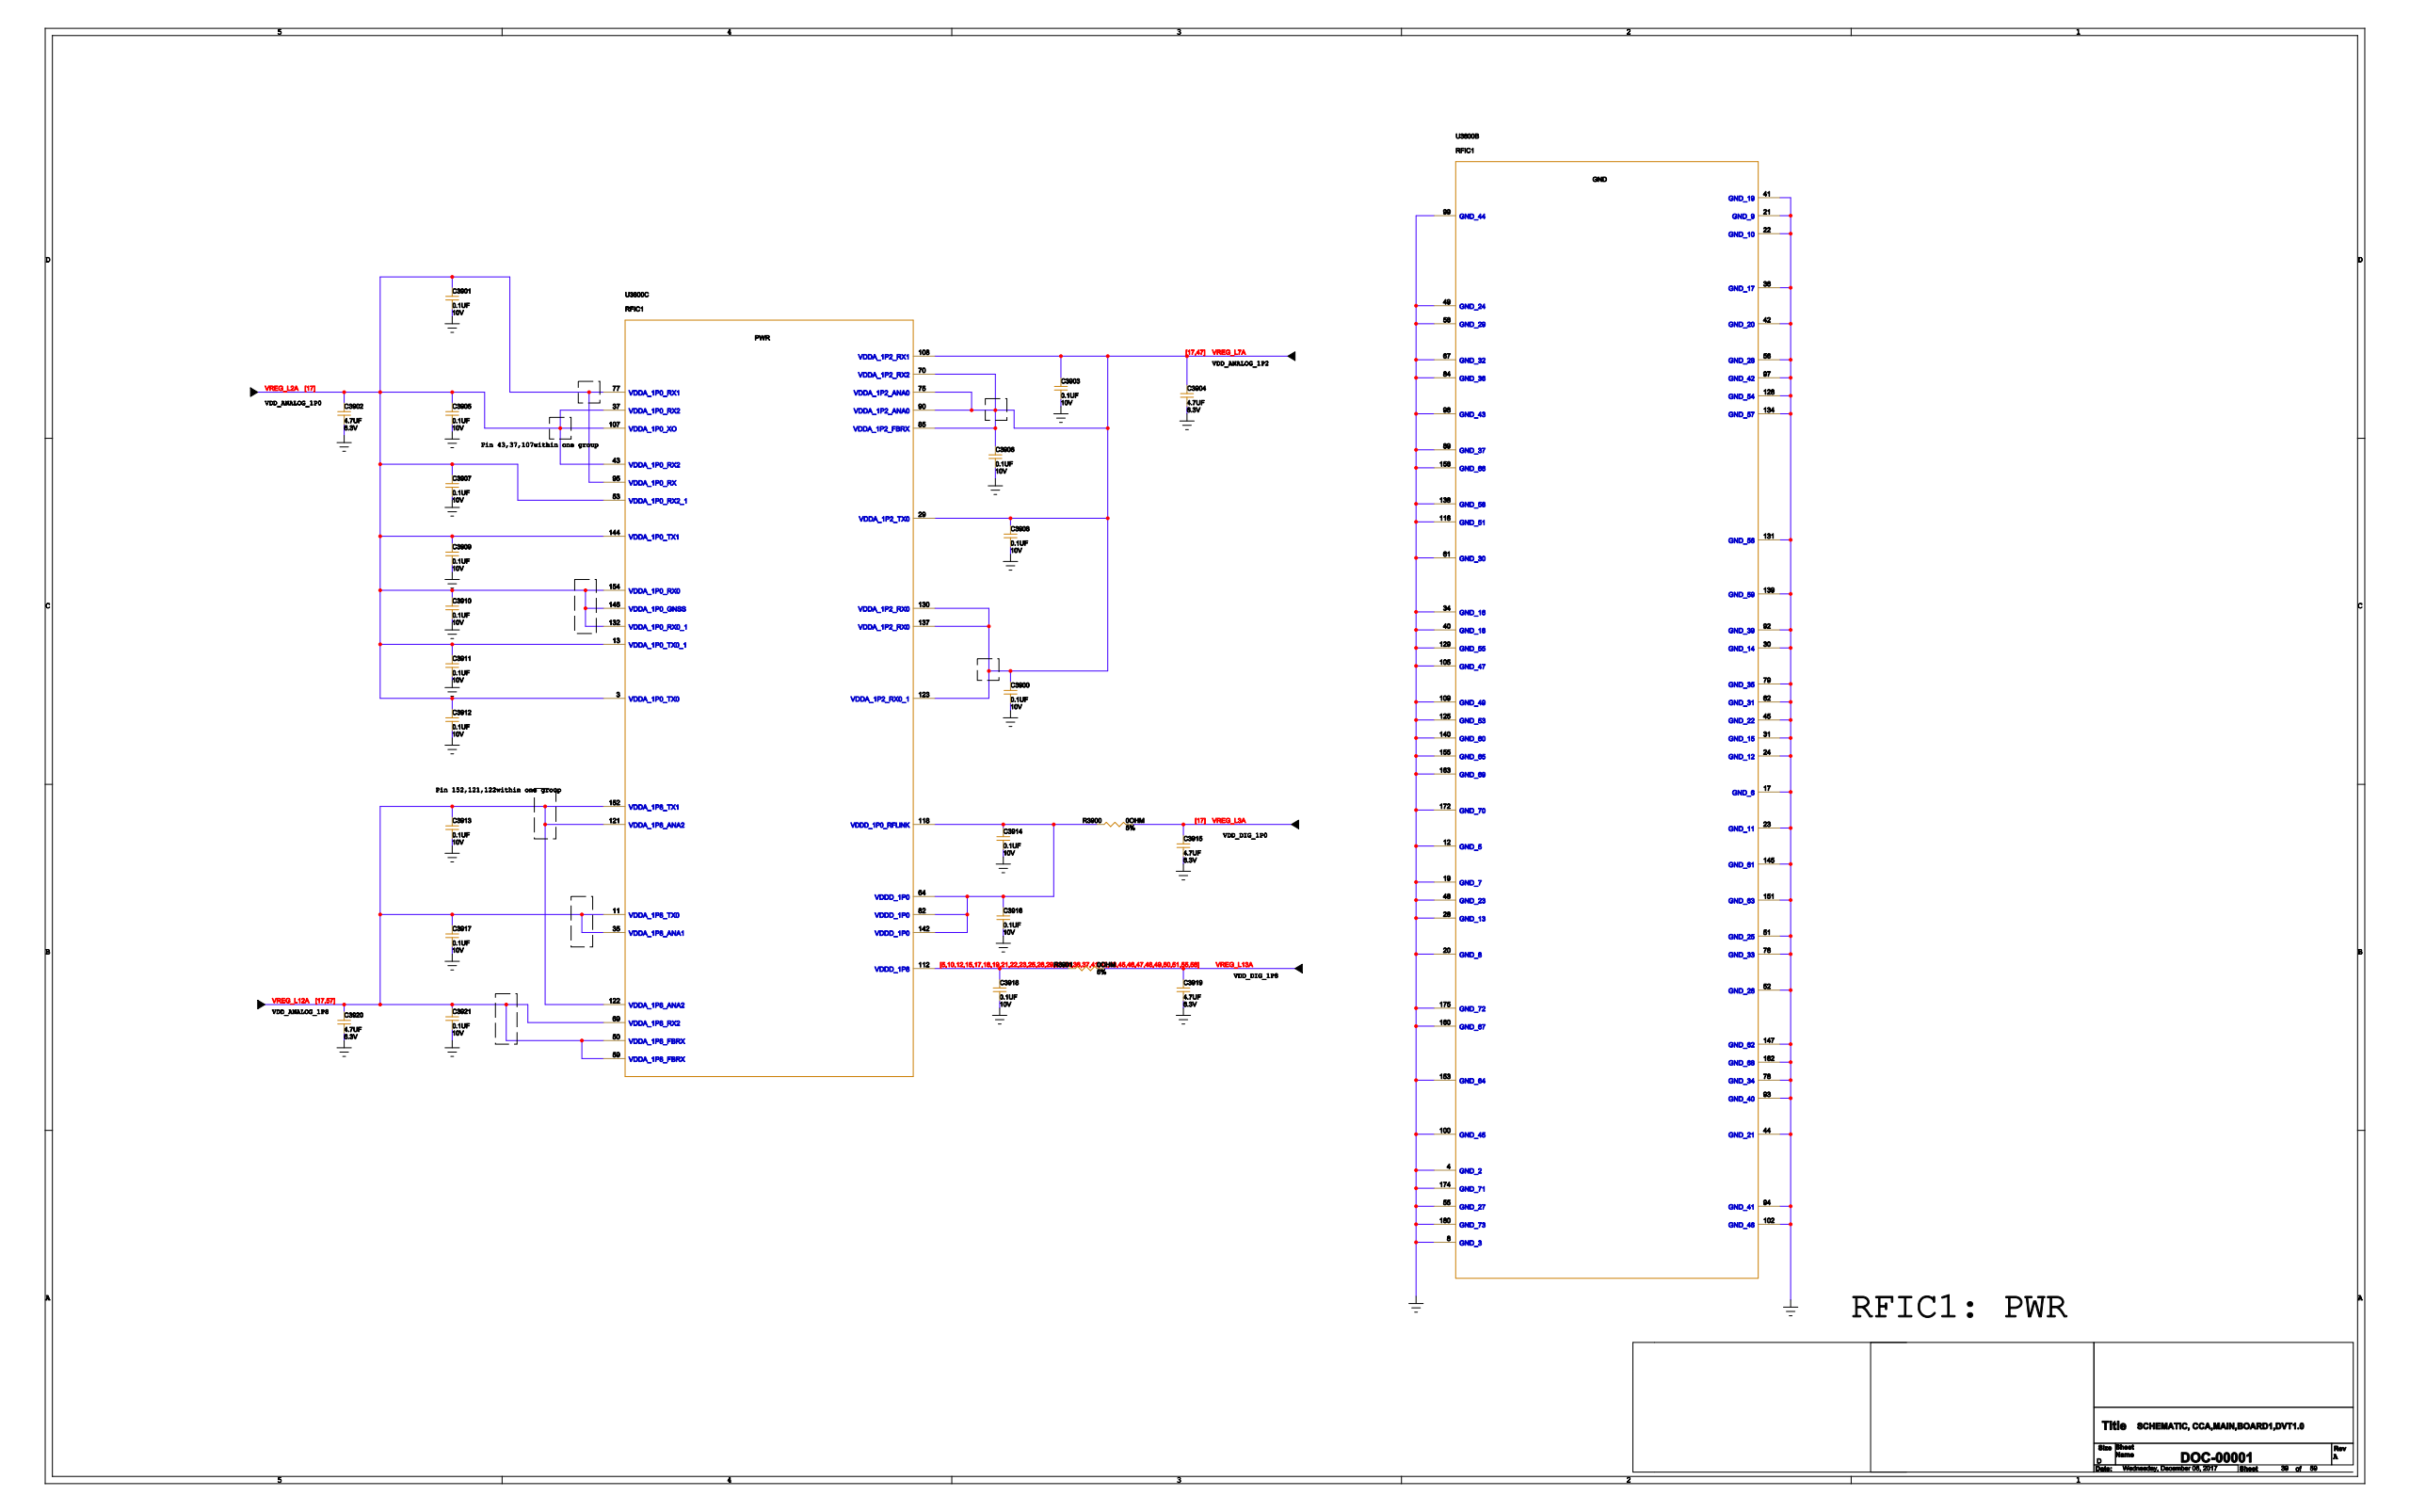Circuit board | KiCad | 1657 parts | 1365 nets | one sheet of the schematic
Parts on this sheet (reference | value | footprint):
C3900
C3901
C3902
C3903
C3904
C3905
C3906
C3907
C3908
C3909
C3910
C3911
C3912
C3913
C3914
C3915
C3916
C3917
C3918
C3919
C3920
C3921
R3900
R3901
U3800
Nets of these parts (net: part-pin ...):
GND: C3900-2 C3901-2 C3902-2 C3903-2 C3904-2 C3905-2 C3906-2 C3907-2 C3908-2 C3909-2 C3910-2 C3911-2 C3912-2 C3913-2 C3914-2 C3915-2 C3916-2 C3917-2 C3918-2 C3919-2 C3920-2 C3921-2 U3800-4 U3800-8 U3800-12 U3800-17 U3800-19 U3800-20 U3800-21 U3800-22 U3800-23 U3800-24 U3800-28 U3800-30 U3800-31 U3800-34 U3800-36 U3800-40 U3800-41 U3800-42 U3800-44 U3800-45 U3800-48 U3800-49 U3800-51 U3800-52 U3800-55 U3800-56 U3800-58 U3800-61 U3800-62 U3800-67 U3800-76 U3800-78 U3800-79 U3800-84 U3800-89 U3800-92 U3800-93 U3800-94 U3800-97 U3800-98 U3800-99 U3800-100 U3800-102 U3800-105 U3800-109 U3800-116 U3800-125 U3800-128 U3800-129 U3800-131 U3800-134 U3800-138 U3800-139 U3800-140 U3800-145 U3800-147 U3800-151 U3800-153 U3800-155 U3800-158 U3800-160 U3800-162 U3800-163 U3800-172 U3800-174 U3800-175 U3800-180
VREG_L13A: C3919-1 R3901-2
VREG_L12A: C3913-1 C3917-1 C3920-1 C3921-1 U3800-11 U3800-35 U3800-50 U3800-59 U3800-69 U3800-121 U3800-122 U3800-152
VREG_L7A: C3900-1 C3903-1 C3904-1 C3906-1 C3908-1 U3800-29 U3800-70 U3800-75 U3800-85 U3800-90 U3800-108 U3800-123 U3800-130 U3800-137
N42470007: C3914-1 C3916-1 R3900-1 U3800-64 U3800-82 U3800-118 U3800-142
VREG_L2A: C3901-1 C3902-1 C3905-1 C3907-1 C3909-1 C3910-1 C3911-1 C3912-1 U3800-3 U3800-13 U3800-37 U3800-43 U3800-53 U3800-77 U3800-95 U3800-107 U3800-132 U3800-144 U3800-146 U3800-154
VREG_L3A: C3915-1 R3900-2
N42469979: C3918-1 R3901-1 U3800-112